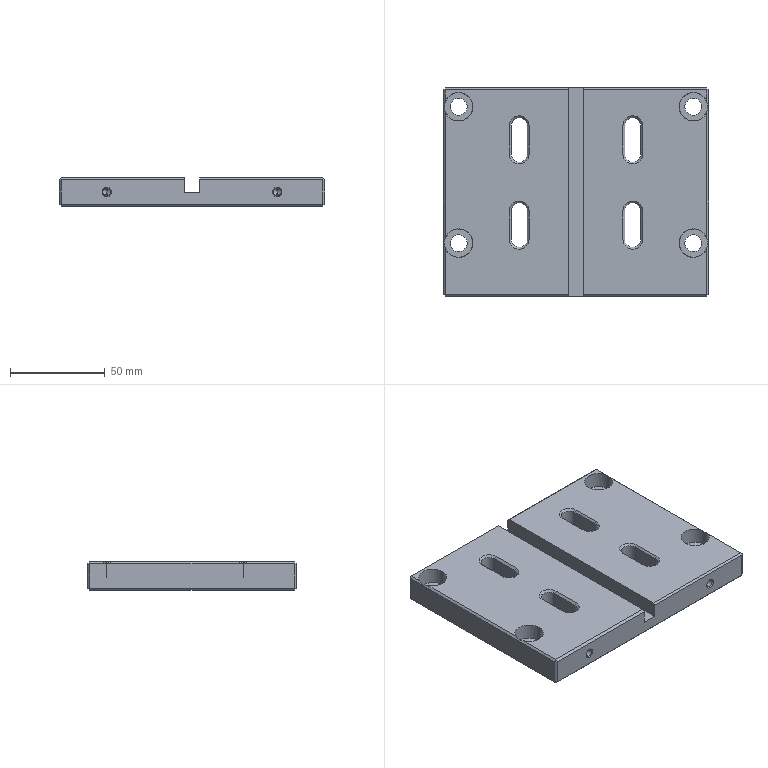Part | SolidWorks | features HoleWzd 3, Chamfer 2, Cut 1, Extrusion 1, ICE 1, LibraryFeature 1 | 1 solid | 112 faces | box 140 x 110 x 15 mm | volume 204135 mm3 | plane 60 | cylinder 28 | cone 24 | commonest cylinder face diameters 8.5 x8 9 x8 15 x8 4.2 x4